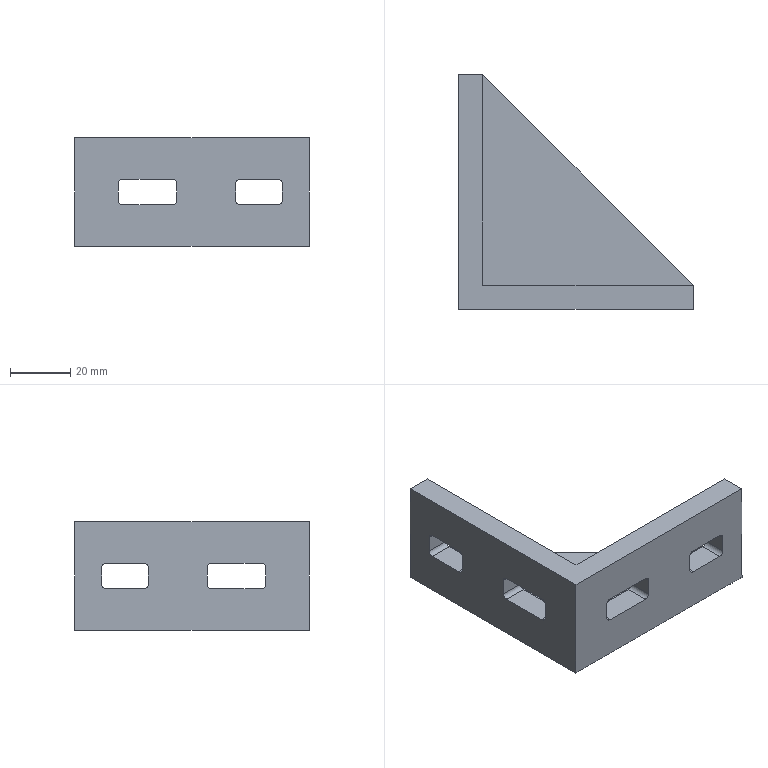Part | STEP file | Die-cast aluminium connector, 40 series, 40mm face, reinforced type | 1 solid | 42 faces | box 78 x 78 x 36 mm | volume 52626 mm3 | plane 26 | cylinder 16 | commonest cylinder face diameters 3 x16